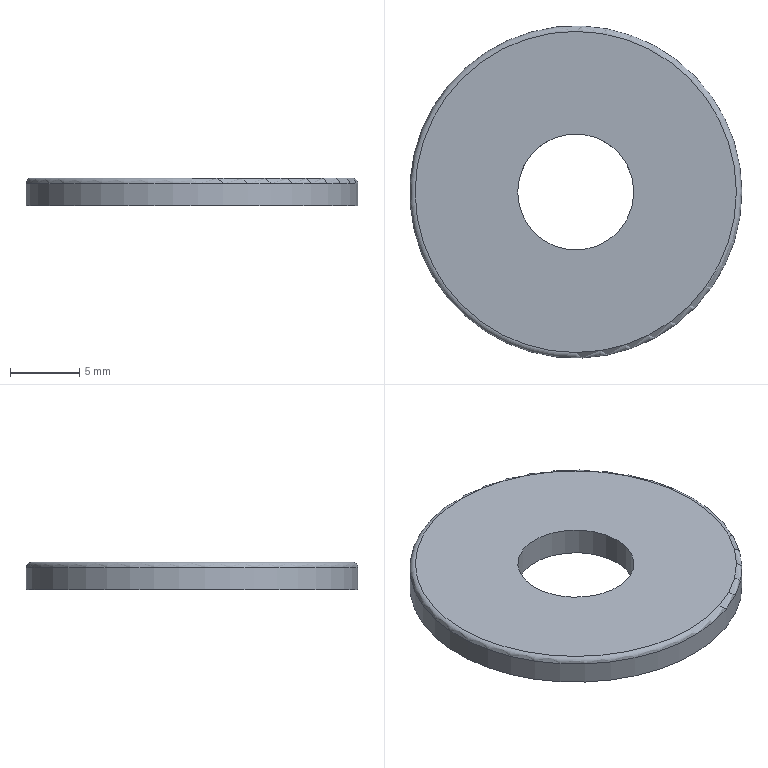Part | STEP file | Frame_lock | 1 solid | 5 faces | box 24 x 24 x 2 mm | volume 791.374 mm3 | cylinder 2 | plane 2 | torus 1 | commonest cylinder face diameters 8.4 x1 24 x1
STEP:
#1=CARTESIAN_POINT('',(0.,0.,0.));
#2=DIRECTION('',(0.,0.,1.));
#3=DIRECTION('',(1.,0.,0.));
#4=AXIS2_PLACEMENT_3D('',#1,#2,#3);
#5=CARTESIAN_POINT('',(12.,0.,0.));
#6=VERTEX_POINT('',#5);
#7=CARTESIAN_POINT('',(0.,0.,0.));
#8=DIRECTION('',(0.,0.,1.));
#9=DIRECTION('',(1.,0.,0.));
#10=AXIS2_PLACEMENT_3D('',#7,#8,#9);
#11=CIRCLE('',#10,12.);
#12=CARTESIAN_POINT('',(0.,0.,0.));
#13=DIRECTION('',(0.,0.,-1.));
#14=DIRECTION('',(1.,0.,0.));
#15=AXIS2_PLACEMENT_3D('',#12,#13,#14);
#16=CYLINDRICAL_SURFACE('',#15,12.);
#17=CARTESIAN_POINT('',(6.283,0.));
#18=DIRECTION('',(-1.,0.));
#19=VECTOR('',#18,1.);
#20=LINE('',#17,#19);
#21=(GEOMETRIC_REPRESENTATION_CONTEXT(2)PARAMETRIC_REPRESENTATION_CONTEXT()REPRESENTATION_CONTEXT('',''));
#22=DEFINITIONAL_REPRESENTATION('',(#20),#21);
#23=PCURVE('',#16,#22);
#24=CARTESIAN_POINT('',(0.,0.,0.));
#25=DIRECTION('',(0.,0.,1.));
#26=DIRECTION('',(1.,0.,0.));
#27=AXIS2_PLACEMENT_3D('',#24,#25,#26);
#28=PLANE('',#27);
#29=CARTESIAN_POINT('',(0.,0.));
#30=DIRECTION('',(1.,0.));
#31=AXIS2_PLACEMENT_2D('',#29,#30);
#32=CIRCLE('',#31,12.);
#33=(GEOMETRIC_REPRESENTATION_CONTEXT(2)PARAMETRIC_REPRESENTATION_CONTEXT()REPRESENTATION_CONTEXT('',''));
#34=DEFINITIONAL_REPRESENTATION('',(#32),#33);
#35=PCURVE('',#28,#34);
#36=SURFACE_CURVE('',#11,(#23,#35),.PCURVE_S1.);
#37=EDGE_CURVE('',#6,#6,#36,.T.);
#38=ORIENTED_EDGE('',*,*,#37,.T.);
#39=CARTESIAN_POINT('',(12.,0.,1.6));
#40=VERTEX_POINT('',#39);
#41=CARTESIAN_POINT('',(12.,0.,0.));
#42=DIRECTION('',(0.,0.,1.));
#43=VECTOR('',#42,1.);
#44=LINE('',#41,#43);
#45=CARTESIAN_POINT('',(0.,0.));
#46=DIRECTION('',(0.,-1.));
#47=VECTOR('',#46,1.);
#48=LINE('',#45,#47);
#49=(GEOMETRIC_REPRESENTATION_CONTEXT(2)PARAMETRIC_REPRESENTATION_CONTEXT()REPRESENTATION_CONTEXT('',''));
#50=DEFINITIONAL_REPRESENTATION('',(#48),#49);
#51=PCURVE('',#16,#50);
#52=CARTESIAN_POINT('',(6.283,0.));
#53=DIRECTION('',(0.,-1.));
#54=VECTOR('',#53,1.);
#55=LINE('',#52,#54);
#56=(GEOMETRIC_REPRESENTATION_CONTEXT(2)PARAMETRIC_REPRESENTATION_CONTEXT()REPRESENTATION_CONTEXT('',''));
#57=DEFINITIONAL_REPRESENTATION('',(#55),#56);
#58=PCURVE('',#16,#57);
#59=SEAM_CURVE('',#44,(#51,#58),.PCURVE_S1.);
#60=EDGE_CURVE('',#6,#40,#59,.T.);
#61=ORIENTED_EDGE('',*,*,#60,.T.);
#62=CARTESIAN_POINT('',(0.,0.,1.6));
#63=DIRECTION('',(0.,0.,1.));
#64=DIRECTION('',(1.,0.,0.));
#65=AXIS2_PLACEMENT_3D('',#62,#63,#64);
#66=CIRCLE('',#65,12.);
#67=CARTESIAN_POINT('',(6.283,-1.6));
#68=DIRECTION('',(-1.,0.));
#69=VECTOR('',#68,1.);
#70=LINE('',#67,#69);
#71=(GEOMETRIC_REPRESENTATION_CONTEXT(2)PARAMETRIC_REPRESENTATION_CONTEXT()REPRESENTATION_CONTEXT('',''));
#72=DEFINITIONAL_REPRESENTATION('',(#70),#71);
#73=PCURVE('',#16,#72);
#74=CARTESIAN_POINT('',(0.,0.,1.6));
#75=DIRECTION('',(0.,0.,1.));
#76=DIRECTION('',(1.,0.,0.));
#77=AXIS2_PLACEMENT_3D('',#74,#75,#76);
#78=TOROIDAL_SURFACE('',#77,11.6,0.4);
#79=CARTESIAN_POINT('',(0.,0.));
#80=DIRECTION('',(1.,0.));
#81=VECTOR('',#80,1.);
#82=LINE('',#79,#81);
#83=(GEOMETRIC_REPRESENTATION_CONTEXT(2)PARAMETRIC_REPRESENTATION_CONTEXT()REPRESENTATION_CONTEXT('',''));
#84=DEFINITIONAL_REPRESENTATION('',(#82),#83);
#85=PCURVE('',#78,#84);
#86=SURFACE_CURVE('',#66,(#73,#85),.PCURVE_S1.);
#87=EDGE_CURVE('',#40,#40,#86,.T.);
#88=ORIENTED_EDGE('',*,*,#87,.F.);
#89=ORIENTED_EDGE('',*,*,#60,.F.);
#90=EDGE_LOOP('',(#38,#61,#88,#89));
#91=FACE_BOUND('',#90,.T.);
#92=ADVANCED_FACE('',(#91),#16,.T.);
#93=CARTESIAN_POINT('',(11.6,0.,2.));
#94=VERTEX_POINT('',#93);
#95=CARTESIAN_POINT('',(11.6,0.,1.6));
#96=DIRECTION('',(0.,-1.,0.));
#97=DIRECTION('',(1.,0.,0.));
#98=AXIS2_PLACEMENT_3D('',#95,#96,#97);
#99=CIRCLE('',#98,0.4);
#100=CARTESIAN_POINT('',(0.,0.));
#101=DIRECTION('',(0.,1.));
#102=VECTOR('',#101,1.);
#103=LINE('',#100,#102);
#104=(GEOMETRIC_REPRESENTATION_CONTEXT(2)PARAMETRIC_REPRESENTATION_CONTEXT()REPRESENTATION_CONTEXT('',''));
#105=DEFINITIONAL_REPRESENTATION('',(#103),#104);
#106=PCURVE('',#78,#105);
#107=CARTESIAN_POINT('',(6.283,0.));
#108=DIRECTION('',(0.,1.));
#109=VECTOR('',#108,1.);
#110=LINE('',#107,#109);
#111=(GEOMETRIC_REPRESENTATION_CONTEXT(2)PARAMETRIC_REPRESENTATION_CONTEXT()REPRESENTATION_CONTEXT('',''));
#112=DEFINITIONAL_REPRESENTATION('',(#110),#111);
#113=PCURVE('',#78,#112);
#114=SEAM_CURVE('',#99,(#106,#113),.PCURVE_S1.);
#115=EDGE_CURVE('',#40,#94,#114,.T.);
#116=ORIENTED_EDGE('',*,*,#115,.F.);
#117=ORIENTED_EDGE('',*,*,#87,.T.);
#118=ORIENTED_EDGE('',*,*,#115,.T.);
#119=CARTESIAN_POINT('',(0.,0.,2.));
#120=DIRECTION('',(0.,0.,1.));
#121=DIRECTION('',(1.,0.,0.));
#122=AXIS2_PLACEMENT_3D('',#119,#120,#121);
#123=CIRCLE('',#122,11.6);
#124=CARTESIAN_POINT('',(0.,1.571));
#125=DIRECTION('',(1.,0.));
#126=VECTOR('',#125,1.);
#127=LINE('',#124,#126);
#128=(GEOMETRIC_REPRESENTATION_CONTEXT(2)PARAMETRIC_REPRESENTATION_CONTEXT()REPRESENTATION_CONTEXT('',''));
#129=DEFINITIONAL_REPRESENTATION('',(#127),#128);
#130=PCURVE('',#78,#129);
#131=CARTESIAN_POINT('',(0.,0.,2.));
#132=DIRECTION('',(0.,0.,1.));
#133=DIRECTION('',(1.,0.,0.));
#134=AXIS2_PLACEMENT_3D('',#131,#132,#133);
#135=PLANE('',#134);
#136=CARTESIAN_POINT('',(0.,0.));
#137=DIRECTION('',(1.,0.));
#138=AXIS2_PLACEMENT_2D('',#136,#137);
#139=CIRCLE('',#138,11.6);
#140=(GEOMETRIC_REPRESENTATION_CONTEXT(2)PARAMETRIC_REPRESENTATION_CONTEXT()REPRESENTATION_CONTEXT('',''));
#141=DEFINITIONAL_REPRESENTATION('',(#139),#140);
#142=PCURVE('',#135,#141);
#143=SURFACE_CURVE('',#123,(#130,#142),.PCURVE_S1.);
#144=EDGE_CURVE('',#94,#94,#143,.T.);
#145=ORIENTED_EDGE('',*,*,#144,.F.);
#146=EDGE_LOOP('',(#116,#117,#118,#145));
#147=FACE_BOUND('',#146,.T.);
#148=ADVANCED_FACE('',(#147),#78,.T.);
#149=ORIENTED_EDGE('',*,*,#37,.T.);
#150=EDGE_LOOP('',(#149));
#151=FACE_BOUND('',#150,.F.);
#152=CARTESIAN_POINT('',(4.2,0.,0.));
#153=VERTEX_POINT('',#152);
#154=CARTESIAN_POINT('',(0.,0.,0.));
#155=DIRECTION('',(0.,0.,1.));
#156=DIRECTION('',(1.,0.,0.));
#157=AXIS2_PLACEMENT_3D('',#154,#155,#156);
#158=CIRCLE('',#157,4.2);
#159=CARTESIAN_POINT('',(0.,0.));
#160=DIRECTION('',(1.,0.));
#161=AXIS2_PLACEMENT_2D('',#159,#160);
#162=CIRCLE('',#161,4.2);
#163=(GEOMETRIC_REPRESENTATION_CONTEXT(2)PARAMETRIC_REPRESENTATION_CONTEXT()REPRESENTATION_CONTEXT('',''));
#164=DEFINITIONAL_REPRESENTATION('',(#162),#163);
#165=PCURVE('',#28,#164);
#166=CARTESIAN_POINT('',(0.,0.,0.));
#167=DIRECTION('',(0.,0.,-1.));
#168=DIRECTION('',(1.,0.,0.));
#169=AXIS2_PLACEMENT_3D('',#166,#167,#168);
#170=CYLINDRICAL_SURFACE('',#169,4.2);
#171=CARTESIAN_POINT('',(6.283,0.));
#172=DIRECTION('',(-1.,0.));
#173=VECTOR('',#172,1.);
#174=LINE('',#171,#173);
#175=(GEOMETRIC_REPRESENTATION_CONTEXT(2)PARAMETRIC_REPRESENTATION_CONTEXT()REPRESENTATION_CONTEXT('',''));
#176=DEFINITIONAL_REPRESENTATION('',(#174),#175);
#177=PCURVE('',#170,#176);
#178=SURFACE_CURVE('',#158,(#165,#177),.PCURVE_S1.);
#179=EDGE_CURVE('',#153,#153,#178,.T.);
#180=ORIENTED_EDGE('',*,*,#179,.T.);
#181=EDGE_LOOP('',(#180));
#182=FACE_BOUND('',#181,.T.);
#183=ADVANCED_FACE('',(#151,#182),#28,.F.);
#184=ORIENTED_EDGE('',*,*,#144,.T.);
#185=EDGE_LOOP('',(#184));
#186=FACE_BOUND('',#185,.T.);
#187=CARTESIAN_POINT('',(4.2,0.,2.));
#188=VERTEX_POINT('',#187);
#189=CARTESIAN_POINT('',(0.,0.,2.));
#190=DIRECTION('',(0.,0.,1.));
#191=DIRECTION('',(1.,0.,0.));
#192=AXIS2_PLACEMENT_3D('',#189,#190,#191);
#193=CIRCLE('',#192,4.2);
#194=CARTESIAN_POINT('',(0.,0.));
#195=DIRECTION('',(1.,0.));
#196=AXIS2_PLACEMENT_2D('',#194,#195);
#197=CIRCLE('',#196,4.2);
#198=(GEOMETRIC_REPRESENTATION_CONTEXT(2)PARAMETRIC_REPRESENTATION_CONTEXT()REPRESENTATION_CONTEXT('',''));
#199=DEFINITIONAL_REPRESENTATION('',(#197),#198);
#200=PCURVE('',#135,#199);
#201=CARTESIAN_POINT('',(6.283,-2.));
#202=DIRECTION('',(-1.,0.));
#203=VECTOR('',#202,1.);
#204=LINE('',#201,#203);
#205=(GEOMETRIC_REPRESENTATION_CONTEXT(2)PARAMETRIC_REPRESENTATION_CONTEXT()REPRESENTATION_CONTEXT('',''));
#206=DEFINITIONAL_REPRESENTATION('',(#204),#205);
#207=PCURVE('',#170,#206);
#208=SURFACE_CURVE('',#193,(#200,#207),.PCURVE_S1.);
#209=EDGE_CURVE('',#188,#188,#208,.T.);
#210=ORIENTED_EDGE('',*,*,#209,.T.);
#211=EDGE_LOOP('',(#210));
#212=FACE_BOUND('',#211,.F.);
#213=ADVANCED_FACE('',(#186,#212),#135,.T.);
#214=ORIENTED_EDGE('',*,*,#179,.T.);
#215=CARTESIAN_POINT('',(4.2,0.,0.));
#216=DIRECTION('',(0.,0.,1.));
#217=VECTOR('',#216,1.);
#218=LINE('',#215,#217);
#219=CARTESIAN_POINT('',(0.,0.));
#220=DIRECTION('',(0.,-1.));
#221=VECTOR('',#220,1.);
#222=LINE('',#219,#221);
#223=(GEOMETRIC_REPRESENTATION_CONTEXT(2)PARAMETRIC_REPRESENTATION_CONTEXT()REPRESENTATION_CONTEXT('',''));
#224=DEFINITIONAL_REPRESENTATION('',(#222),#223);
#225=PCURVE('',#170,#224);
#226=CARTESIAN_POINT('',(6.283,0.));
#227=DIRECTION('',(0.,-1.));
#228=VECTOR('',#227,1.);
#229=LINE('',#226,#228);
#230=(GEOMETRIC_REPRESENTATION_CONTEXT(2)PARAMETRIC_REPRESENTATION_CONTEXT()REPRESENTATION_CONTEXT('',''));
#231=DEFINITIONAL_REPRESENTATION('',(#229),#230);
#232=PCURVE('',#170,#231);
#233=SEAM_CURVE('',#218,(#225,#232),.PCURVE_S1.);
#234=EDGE_CURVE('',#153,#188,#233,.T.);
#235=ORIENTED_EDGE('',*,*,#234,.T.);
#236=ORIENTED_EDGE('',*,*,#209,.F.);
#237=ORIENTED_EDGE('',*,*,#234,.F.);
#238=EDGE_LOOP('',(#214,#235,#236,#237));
#239=FACE_BOUND('',#238,.F.);
#240=ADVANCED_FACE('',(#239),#170,.F.);
#241=CLOSED_SHELL('',(#92,#148,#183,#213,#240));
#242=MANIFOLD_SOLID_BREP('',#241);
#243=(LENGTH_UNIT()NAMED_UNIT(*)SI_UNIT(.MILLI.,.METRE.));
#244=UNCERTAINTY_MEASURE_WITH_UNIT(LENGTH_MEASURE(0.0000001),#243,'','');
#245=(NAMED_UNIT(*)PLANE_ANGLE_UNIT()SI_UNIT($,.RADIAN.));
#246=(NAMED_UNIT(*)SI_UNIT($,.STERADIAN.)SOLID_ANGLE_UNIT());
#247=(GEOMETRIC_REPRESENTATION_CONTEXT(3)GLOBAL_UNCERTAINTY_ASSIGNED_CONTEXT((#244))GLOBAL_UNIT_ASSIGNED_CONTEXT((#243,#245,#246))REPRESENTATION_CONTEXT('',''));
#248=ADVANCED_BREP_SHAPE_REPRESENTATION('',(#4,#242),#247);